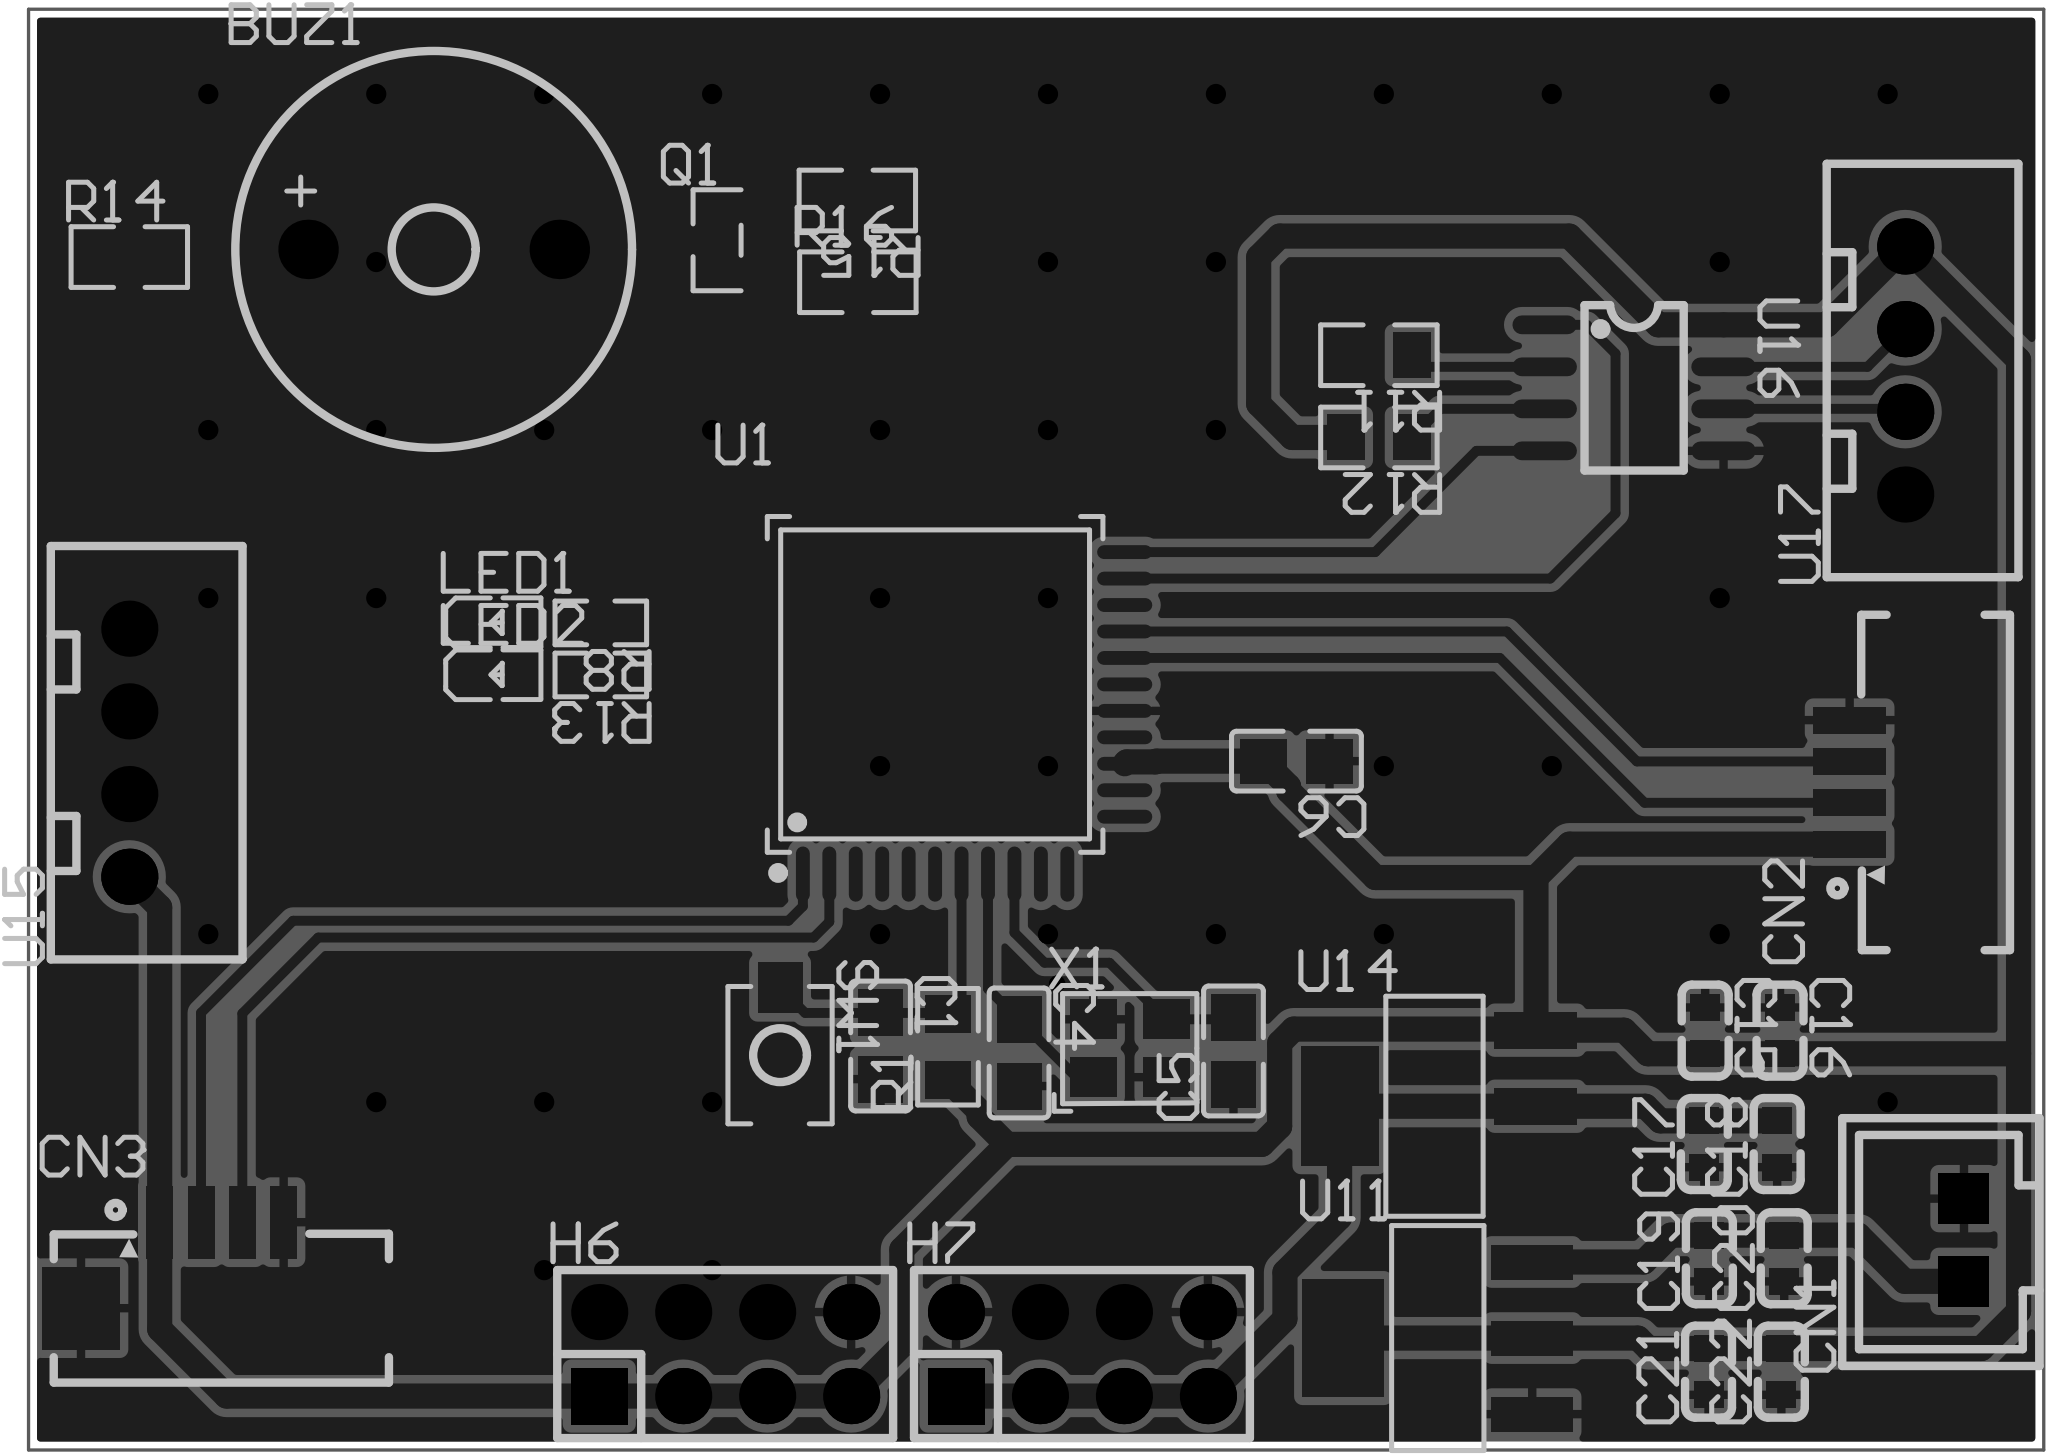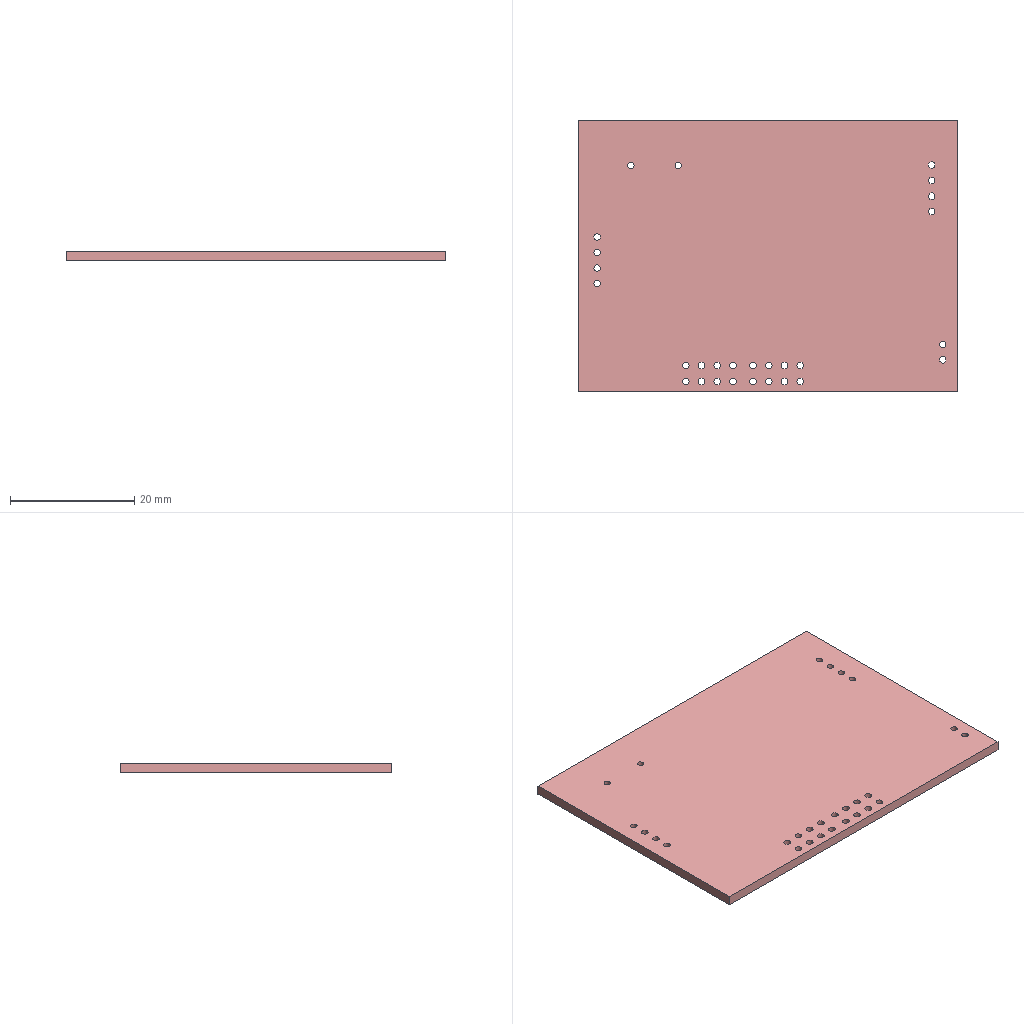Circuit board layout | Altium Designer | box 61 x 43.6 x 1.6 mm
Layer stack:
# Altium Designer layer stack of  (unit mm; dielectric type: 0 none, 1 core, 2 prepreg, 3 surface material)
index,name,kind,layer,copper_thickness_mm,dielectric_type,dielectric_thickness_mm,dielectric_material,dielectric_constant
0,Top Paste Mask Layer,other,,,,,,
1,Top Silkscreen Layer,other,,,,,,
2,Top Solder Mask Layer,dielectric,,,3,0.01,,3.3
3,Top Layer,copper,Top Layer,0.035,,,,
4,Dielectric1,dielectric,,,3,1.51,FR4,4.5
5,Bottom Layer,copper,Bottom Layer,0.035,,,,
6,Bottom Solder Mask Layer,dielectric,,,3,0.01,,3.3
7,Bottom Silkscreen Layer,other,,,,,,
8,Bottom Paste Mask Layer,other,,,,,,
# drill layer pairs: low layer,high layer
drill_pair,Top Layer,Bottom Layer
Part placement:
Designator,Comment,Layer,Footprint,Center-X(mm),Center-Y(mm),Rotation
BUZ1,5VDC???,F12,??7.6,TopLayer,BUZ-TH_BD12.0-P7.60-D0.6-FD,97.472,122.532,0
C1,10uf,TopLayer,C0805,110.99,98.447,270
C4,22pf,TopLayer,C0805,115.181,98.237,270
C5,22pf,TopLayer,C0805,121.666,98.298,90
C6,100nF,TopLayer,C0805,123.571,107.061,180
C15,100nF,TopLayer,C0603,135.935,98.913,270
C16,10uF,TopLayer,C0603,138.199,98.913,270
C17,100nF,TopLayer,C0603,135.909,95.484,90
C18,10uF,TopLayer,C0603,138.112,95.484,90
C19,100nF,TopLayer,C0603,136.062,92.03,90
C20,10uF,TopLayer,C0603,138.326,92.03,90
C21,100nF,TopLayer,C0603,136.036,88.601,90
C22,10uF,TopLayer,C0603,138.239,88.601,90
CN1,XH2.54,TopLayer,CONN-TH_XH2.54-2P,143.764,92.583,90
CN2,HC-1.25-4PWT,TopLayer,CONN-SMD_4P-P1.25-HC-1.25-4PWT,141.605,106.426,90
CN3,HC-1.25-4PWT,TopLayer,CONN-SMD_4P-P1.25-HC-1.25-4PWT,91.059,91.821,0
H6,,TopLayer,HDR-TH_8P-P2.54-V-M-R2-C4-S2.54,106.29,89.134,0
H7,,TopLayer,HDR-TH_8P-P2.54-V-M-R2-C4-S2.54,117.082,89.134,0
LED1,KT-0603R,TopLayer,LED0603-RD,99.326,111.24,0
LED2,KT-0603R,TopLayer,LED0603-RD,99.326,109.666,0
Q1,MMBT4401Q,TopLayer,SOT-23-3_L2.9-W1.3-P1.90-LS2.4-BR,106.045,122.809,0
R1,10K,TopLayer,R0805,113.03,98.425,90
R8,510,TopLayer,R0603,102.528,111.24,180
R11,10K,TopLayer,R0805,126.065,119.333,180
R12,10K,TopLayer,R0805,126.065,116.847,180
R13,510,TopLayer,R0603,102.528,109.666,180
R14,100R,TopLayer,R0805,88.265,122.301,0
R15,100R,TopLayer,R0805,110.288,124.011,180
R16,100R,TopLayer,R0805,110.304,121.54,0
SW1,,TopLayer,Key_SMD_3x4x2,107.95,98.171,270
U1,STC8A8K48D4-45I-LQFP44,TopLayer,LQFP-44_L10.0-W10.0-P0.80-LS12.0-BL,112.641,109.38,0
U11,AMS1117-5.0,TopLayer,SOT-223_L6.5-W3.5-P2.30-LS7.0-BR,127.846,89.617,0
U14,AMS1117-3.3,TopLayer,SOT-223-3_L6.5-W3.4-P2.30-LS7.0-BR,127.846,96.627,0
U15,XH2.54_4P_直插,TopLayer,CONN-TH_4P-P2.50-XH2.54-4P,88.265,107.315,90
U16,SP485EEN-L/TR,TopLayer,SOIC-8_L5.0-W4.0-P1.27-LS6.0-BL,133.785,118.347,270
U17,XH2.54_4P_直插,TopLayer,CONN-TH_4P-P2.50-XH2.54-4P,141.986,118.872,90
X1,12MHz,TopLayer,OSC-SMD_4P-L3.2-W2.5-BL,118.526,98.38,0
Pad and via stacks:
# Altium Designer via and pad stacks of  (unit mm). Each distinct definition once, with the count of objects using it.
# via: kind,start_layer,end_layer,hole_mm,diameter_mm,mode(0 simple;1 top-mid-bottom;2 full stack),diameter_per_layer,count,example_net
# pad: kind,layer,hole_mm,hole_type(0 round;1 square;2 slot),plating,top_size,top_shape(1 round;2 rect;3 octagon;9 rounded rect),mid_size,bottom_size,mode,footprint,size_per_layer,count,example
pad,Multi-Layer,1,0,plated,1.8x1.8,1,1.8x1.8,1.8x1.8,0,BUZ-TH_BD12.0-P7.60-D0.6-FD,,2,BUZ1.2
pad,Multi-Layer,1,2,plated,1.524x1.524,2,1.524x1.524,1.524x1.524,0,CONN-TH_XH2.54-2P,,2,CN1.1
pad,Multi-Layer,1.1,0,plated,1.7x1.7,2,1.7x1.7,1.7x1.7,0,HDR-TH_8P-P2.54-V-M-R2-C4-S2.54,,2,H6.1
pad,Multi-Layer,1.1,0,plated,1.7x1.7,1,1.7x1.7,1.7x1.7,0,HDR-TH_8P-P2.54-V-M-R2-C4-S2.54,,14,H6.2
pad,Multi-Layer,1.05,0,plated,1.7x1.7,1,1.7x1.7,1.7x1.7,0,CONN-TH_4P-P2.50-XH2.54-4P,,8,U15.1
pad,Top Layer,0,0,plated,1.41x1.35,2,1.41x1.35,1.41x1.35,0,C0805,,8,C1.2
pad,Top Layer,0,0,plated,0.8x0.9,2,0.8x0.9,0.8x0.9,0,C0603,,16,C15.2
pad,Top Layer,0,0,plated,2.2x0.8,2,2.2x0.8,2.2x0.8,0,CONN-SMD_4P-P1.25-HC-1.25-4PWT,,8,CN2.1
pad,Top Layer,0,0,plated,2.35x2.5,2,2.35x2.5,2.35x2.5,0,CONN-SMD_4P-P1.25-HC-1.25-4PWT,,4,CN2.5
pad,Top Layer,0,0,plated,0.8x0.8,2,0.8x0.8,0.8x0.8,0,LED0603-RD,,4,LED1.2
pad,Top Layer,0,0,plated,1.25x0.7,2,1.25x0.7,1.25x0.7,0,SOT-23-3_L2.9-W1.3-P1.90-LS2.4-BR,,3,Q1.1
pad,Top Layer,0,0,plated,1.133x1.377,2,1.133x1.377,1.133x1.377,0,R0805,,12,R1.2
pad,Top Layer,0,0,plated,0.8065x0.864,2,0.8065x0.864,0.8065x0.864,0,R0603,,4,R8.2
pad,Top Layer,0,0,plated,1.53x1.36,2,1.53x1.36,1.53x1.36,0,Key_SMD_3x4x2,,2,SW1.1
pad,Top Layer,0,0,plated,0.42x1.67,1,0.42x1.67,0.42x1.67,0,LQFP-44_L10.0-W10.0-P0.80-LS12.0-BL,,22,U1.1
pad,Top Layer,0,0,plated,1.67x0.42,1,1.67x0.42,1.67x0.42,0,LQFP-44_L10.0-W10.0-P0.80-LS12.0-BL,,22,U1.12
pad,Top Layer,0,0,plated,2.465x1.05,2,2.465x1.05,2.465x1.05,0,SOT-223_L6.5-W3.5-P2.30-LS7.0-BR,,3,U11.1
pad,Top Layer,0,0,plated,2.465x3.54,2,2.465x3.54,2.465x3.54,0,SOT-223_L6.5-W3.5-P2.30-LS7.0-BR,,1,U11.4
pad,Top Layer,0,0,plated,2.5x1.1,2,2.5x1.1,2.5x1.1,0,SOT-223-3_L6.5-W3.4-P2.30-LS7.0-BR,,3,U14.1
pad,Top Layer,0,0,plated,2.34x3.6,2,2.34x3.6,2.34x3.6,0,SOT-223-3_L6.5-W3.4-P2.30-LS7.0-BR,,1,U14.4
pad,Top Layer,0,0,plated,0.5684x1.95,1,0.5684x1.95,0.5684x1.95,0,SOIC-8_L5.0-W4.0-P1.27-LS6.0-BL,,8,U16.1
pad,Top Layer,0,0,plated,1.4x1.2,2,1.4x1.2,1.4x1.2,0,OSC-SMD_4P-L3.2-W2.5-BL,,4,X1.1
via,Top Layer,Bottom Layer,0.3048,0.61,0,,43,GND
via,Top Layer,Bottom Layer,0.2997,0.5,0,,1,GND
Copper pours:
name,layer,net,type(0 solid;1 hatched;2 none)
Top Layer-GND,Top Layer,GND,0
Bottom Layer-GND,Bottom Layer,GND,0